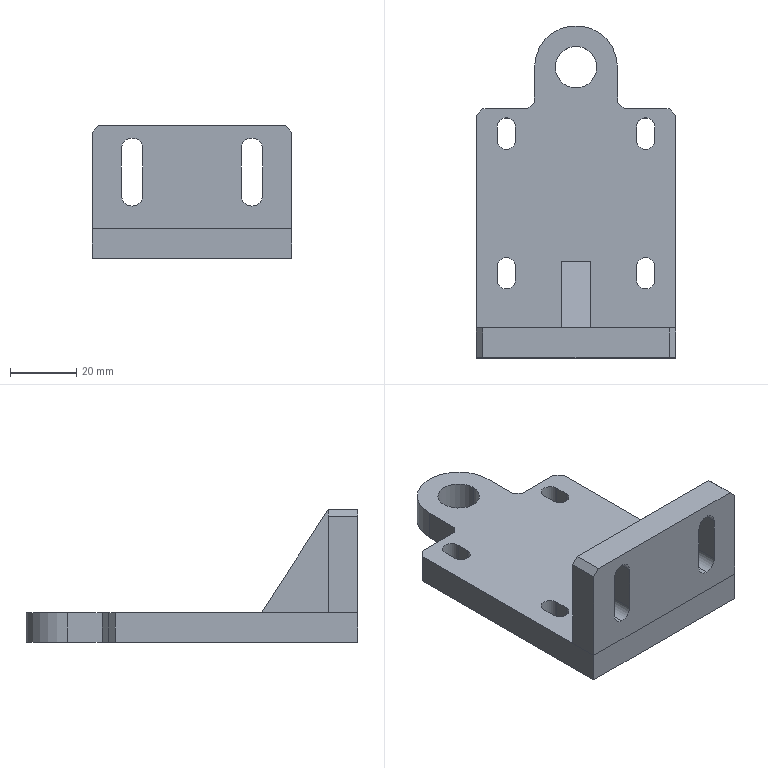Part | STEP file | PN_0022 Rodless cylinder support plate_default_machined_ | 3 solids | 55 faces | box 60 x 100 x 40 mm | volume 60028 mm3 | plane 38 | cylinder 17 | commonest cylinder face diameters 5.5 x8 6.5 x6 12.5 x2 25 x1